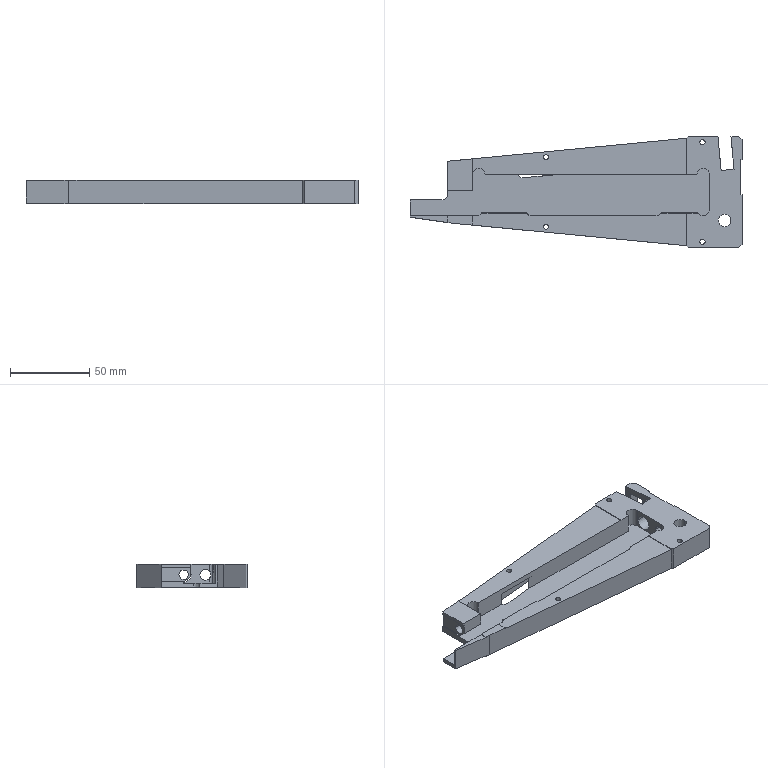Part | SolidWorks | features ICE 13, Chamfer 2, Fillet 2, HoleWzd 2, Extrusion 1 | 1 solid | 99 faces | box 210 x 70 x 15 mm | volume 86149 mm3 | plane 65 | cylinder 34 | commonest cylinder face diameters 8 x11 3.3 x10 6 x5 2.5 x2 7 x2 9.5 x2